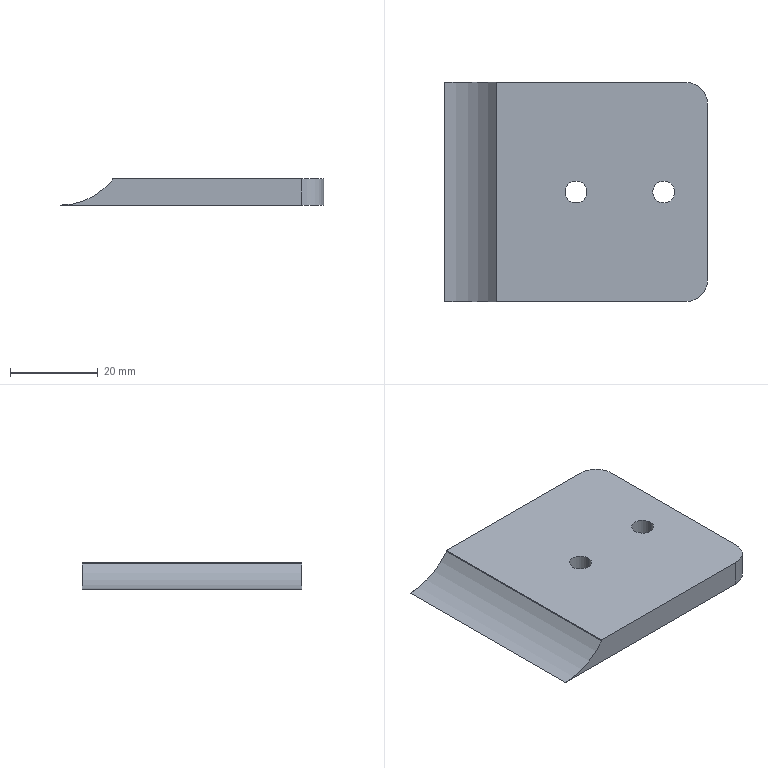Part | SolidWorks | features 3DProfileFeature 1, Extrusion 1, HoleWzd 1, ICE 1 | 1 solid | 13 faces | box 60 x 50 x 6 mm | volume 15185 mm3 | cylinder 7 | plane 6 | commonest cylinder face diameters 5 x4 10 x2 30 x1
STEP:
#1=CARTESIAN_POINT('',(52.5,-30.,-15.));
#2=VERTEX_POINT('',#1);
#3=CARTESIAN_POINT('',(47.5,-30.,-15.));
#4=VERTEX_POINT('',#3);
#5=CARTESIAN_POINT('',(50.,-30.,-15.));
#6=DIRECTION('',(0.,0.,-1.));
#7=DIRECTION('',(-1.,0.,0.));
#8=AXIS2_PLACEMENT_3D('',#5,#6,#7);
#9=CIRCLE('',#8,2.5);
#10=EDGE_CURVE('',#2,#4,#9,.T.);
#11=ORIENTED_EDGE('',*,*,#10,.T.);
#12=CARTESIAN_POINT('',(47.5,-30.,-9.));
#13=VERTEX_POINT('',#12);
#14=CARTESIAN_POINT('',(47.5,-30.,-9.));
#15=DIRECTION('',(0.,0.,1.));
#16=VECTOR('',#15,1000.);
#17=LINE('',#14,#16);
#18=EDGE_CURVE('',#4,#13,#17,.T.);
#19=ORIENTED_EDGE('',*,*,#18,.T.);
#20=CARTESIAN_POINT('',(52.5,-30.,-9.));
#21=VERTEX_POINT('',#20);
#22=CARTESIAN_POINT('',(50.,-30.,-9.));
#23=DIRECTION('',(0.,0.,1.));
#24=DIRECTION('',(1.,0.,0.));
#25=AXIS2_PLACEMENT_3D('',#22,#23,#24);
#26=CIRCLE('',#25,2.5);
#27=EDGE_CURVE('',#13,#21,#26,.T.);
#28=ORIENTED_EDGE('',*,*,#27,.T.);
#29=CARTESIAN_POINT('',(52.5,-30.,-9.));
#30=DIRECTION('',(0.,0.,1.));
#31=VECTOR('',#30,1000.);
#32=LINE('',#29,#31);
#33=EDGE_CURVE('',#2,#21,#32,.T.);
#34=ORIENTED_EDGE('',*,*,#33,.F.);
#35=EDGE_LOOP('',(#11,#19,#28,#34));
#36=FACE_OUTER_BOUND('',#35,.T.);
#37=CARTESIAN_POINT('',(50.,-30.,-9.));
#38=DIRECTION('',(0.,0.,1.));
#39=DIRECTION('',(1.,0.,0.));
#40=AXIS2_PLACEMENT_3D('',#37,#38,#39);
#41=CYLINDRICAL_SURFACE('',#40,2.5);
#42=ADVANCED_FACE('',(#36),#41,.F.);
#43=CARTESIAN_POINT('',(32.5,-30.,-15.));
#44=VERTEX_POINT('',#43);
#45=CARTESIAN_POINT('',(27.5,-30.,-15.));
#46=VERTEX_POINT('',#45);
#47=CARTESIAN_POINT('',(30.,-30.,-15.));
#48=DIRECTION('',(0.,0.,-1.));
#49=DIRECTION('',(-1.,0.,0.));
#50=AXIS2_PLACEMENT_3D('',#47,#48,#49);
#51=CIRCLE('',#50,2.5);
#52=EDGE_CURVE('',#44,#46,#51,.T.);
#53=ORIENTED_EDGE('',*,*,#52,.T.);
#54=CARTESIAN_POINT('',(27.5,-30.,-9.));
#55=VERTEX_POINT('',#54);
#56=CARTESIAN_POINT('',(27.5,-30.,-9.));
#57=DIRECTION('',(0.,0.,1.));
#58=VECTOR('',#57,1000.);
#59=LINE('',#56,#58);
#60=EDGE_CURVE('',#46,#55,#59,.T.);
#61=ORIENTED_EDGE('',*,*,#60,.T.);
#62=CARTESIAN_POINT('',(32.5,-30.,-9.));
#63=VERTEX_POINT('',#62);
#64=CARTESIAN_POINT('',(30.,-30.,-9.));
#65=DIRECTION('',(0.,0.,1.));
#66=DIRECTION('',(1.,0.,0.));
#67=AXIS2_PLACEMENT_3D('',#64,#65,#66);
#68=CIRCLE('',#67,2.5);
#69=EDGE_CURVE('',#55,#63,#68,.T.);
#70=ORIENTED_EDGE('',*,*,#69,.T.);
#71=CARTESIAN_POINT('',(32.5,-30.,-9.));
#72=DIRECTION('',(0.,0.,1.));
#73=VECTOR('',#72,1000.);
#74=LINE('',#71,#73);
#75=EDGE_CURVE('',#44,#63,#74,.T.);
#76=ORIENTED_EDGE('',*,*,#75,.F.);
#77=EDGE_LOOP('',(#53,#61,#70,#76));
#78=FACE_OUTER_BOUND('',#77,.T.);
#79=CARTESIAN_POINT('',(30.,-30.,-9.));
#80=DIRECTION('',(0.,0.,1.));
#81=DIRECTION('',(1.,0.,0.));
#82=AXIS2_PLACEMENT_3D('',#79,#80,#81);
#83=CYLINDRICAL_SURFACE('',#82,2.5);
#84=ADVANCED_FACE('',(#78),#83,.F.);
#85=CARTESIAN_POINT('',(11.8,-55.,-9.261));
#86=VERTEX_POINT('',#85);
#87=CARTESIAN_POINT('',(11.8,-5.,-9.261));
#88=VERTEX_POINT('',#87);
#89=CARTESIAN_POINT('',(11.8,-68.122,-9.261));
#90=DIRECTION('',(0.,1.,0.));
#91=VECTOR('',#90,1000.);
#92=LINE('',#89,#91);
#93=EDGE_CURVE('',#86,#88,#92,.T.);
#94=ORIENTED_EDGE('',*,*,#93,.F.);
#95=CARTESIAN_POINT('',(11.8,-55.,-9.));
#96=VERTEX_POINT('',#95);
#97=CARTESIAN_POINT('',(11.8,-55.,-9.));
#98=DIRECTION('',(0.,0.,-1.));
#99=VECTOR('',#98,1000.);
#100=LINE('',#97,#99);
#101=EDGE_CURVE('',#96,#86,#100,.T.);
#102=ORIENTED_EDGE('',*,*,#101,.F.);
#103=CARTESIAN_POINT('',(11.8,-5.,-9.));
#104=VERTEX_POINT('',#103);
#105=CARTESIAN_POINT('',(11.8,-5.,-9.));
#106=DIRECTION('',(0.,-1.,0.));
#107=VECTOR('',#106,1000.);
#108=LINE('',#105,#107);
#109=EDGE_CURVE('',#104,#96,#108,.T.);
#110=ORIENTED_EDGE('',*,*,#109,.F.);
#111=CARTESIAN_POINT('',(11.8,-5.,-9.));
#112=DIRECTION('',(0.,0.,-1.));
#113=VECTOR('',#112,1000.);
#114=LINE('',#111,#113);
#115=EDGE_CURVE('',#104,#88,#114,.T.);
#116=ORIENTED_EDGE('',*,*,#115,.T.);
#117=EDGE_LOOP('',(#94,#102,#110,#116));
#118=FACE_OUTER_BOUND('',#117,.T.);
#119=CARTESIAN_POINT('',(11.8,-5.,-9.));
#120=DIRECTION('',(1.,0.,0.));
#121=DIRECTION('',(0.,1.,0.));
#122=AXIS2_PLACEMENT_3D('',#119,#120,#121);
#123=PLANE('',#122);
#124=ADVANCED_FACE('',(#118),#123,.F.);
#125=CARTESIAN_POINT('',(0.,-55.,-15.));
#126=VERTEX_POINT('',#125);
#127=CARTESIAN_POINT('',(55.,-55.,-15.));
#128=VERTEX_POINT('',#127);
#129=CARTESIAN_POINT('',(11.8,-55.,-15.));
#130=DIRECTION('',(1.,0.,0.));
#131=VECTOR('',#130,1000.);
#132=LINE('',#129,#131);
#133=EDGE_CURVE('',#126,#128,#132,.T.);
#134=ORIENTED_EDGE('',*,*,#133,.T.);
#135=CARTESIAN_POINT('',(55.,-55.,-9.));
#136=VERTEX_POINT('',#135);
#137=CARTESIAN_POINT('',(55.,-55.,-9.));
#138=DIRECTION('',(0.,0.,-1.));
#139=VECTOR('',#138,1000.);
#140=LINE('',#137,#139);
#141=EDGE_CURVE('',#136,#128,#140,.T.);
#142=ORIENTED_EDGE('',*,*,#141,.F.);
#143=CARTESIAN_POINT('',(11.8,-55.,-9.));
#144=DIRECTION('',(1.,0.,0.));
#145=VECTOR('',#144,1000.);
#146=LINE('',#143,#145);
#147=EDGE_CURVE('',#96,#136,#146,.T.);
#148=ORIENTED_EDGE('',*,*,#147,.F.);
#149=ORIENTED_EDGE('',*,*,#101,.T.);
#150=CARTESIAN_POINT('',(0.,-55.,0.));
#151=DIRECTION('',(0.,1.,0.));
#152=DIRECTION('',(0.,0.,1.));
#153=AXIS2_PLACEMENT_3D('',#150,#151,#152);
#154=CIRCLE('',#153,15.);
#155=EDGE_CURVE('',#86,#126,#154,.T.);
#156=ORIENTED_EDGE('',*,*,#155,.T.);
#157=EDGE_LOOP('',(#134,#142,#148,#149,#156));
#158=FACE_OUTER_BOUND('',#157,.T.);
#159=CARTESIAN_POINT('',(11.8,-55.,-9.));
#160=DIRECTION('',(0.,1.,0.));
#161=DIRECTION('',(0.,0.,1.));
#162=AXIS2_PLACEMENT_3D('',#159,#160,#161);
#163=PLANE('',#162);
#164=ADVANCED_FACE('',(#158),#163,.F.);
#165=CARTESIAN_POINT('',(60.,-50.,-15.));
#166=VERTEX_POINT('',#165);
#167=CARTESIAN_POINT('',(55.,-50.,-15.));
#168=DIRECTION('',(0.,0.,1.));
#169=DIRECTION('',(-1.,0.,0.));
#170=AXIS2_PLACEMENT_3D('',#167,#168,#169);
#171=CIRCLE('',#170,5.);
#172=EDGE_CURVE('',#128,#166,#171,.T.);
#173=ORIENTED_EDGE('',*,*,#172,.T.);
#174=CARTESIAN_POINT('',(60.,-50.,-9.));
#175=VERTEX_POINT('',#174);
#176=CARTESIAN_POINT('',(60.,-50.,-9.));
#177=DIRECTION('',(0.,0.,-1.));
#178=VECTOR('',#177,1000.);
#179=LINE('',#176,#178);
#180=EDGE_CURVE('',#175,#166,#179,.T.);
#181=ORIENTED_EDGE('',*,*,#180,.F.);
#182=CARTESIAN_POINT('',(55.,-50.,-9.));
#183=DIRECTION('',(0.,0.,1.));
#184=DIRECTION('',(-1.,0.,0.));
#185=AXIS2_PLACEMENT_3D('',#182,#183,#184);
#186=CIRCLE('',#185,5.);
#187=EDGE_CURVE('',#136,#175,#186,.T.);
#188=ORIENTED_EDGE('',*,*,#187,.F.);
#189=ORIENTED_EDGE('',*,*,#141,.T.);
#190=EDGE_LOOP('',(#173,#181,#188,#189));
#191=FACE_OUTER_BOUND('',#190,.T.);
#192=CARTESIAN_POINT('',(55.,-50.,-9.));
#193=DIRECTION('',(0.,0.,-1.));
#194=DIRECTION('',(-1.,0.,0.));
#195=AXIS2_PLACEMENT_3D('',#192,#193,#194);
#196=CYLINDRICAL_SURFACE('',#195,5.);
#197=ADVANCED_FACE('',(#191),#196,.T.);
#198=CARTESIAN_POINT('',(60.,-10.,-15.));
#199=VERTEX_POINT('',#198);
#200=CARTESIAN_POINT('',(60.,-10.,-15.));
#201=DIRECTION('',(0.,1.,0.));
#202=VECTOR('',#201,1000.);
#203=LINE('',#200,#202);
#204=EDGE_CURVE('',#166,#199,#203,.T.);
#205=ORIENTED_EDGE('',*,*,#204,.T.);
#206=CARTESIAN_POINT('',(60.,-10.,-9.));
#207=VERTEX_POINT('',#206);
#208=CARTESIAN_POINT('',(60.,-10.,-9.));
#209=DIRECTION('',(0.,0.,-1.));
#210=VECTOR('',#209,1000.);
#211=LINE('',#208,#210);
#212=EDGE_CURVE('',#207,#199,#211,.T.);
#213=ORIENTED_EDGE('',*,*,#212,.F.);
#214=CARTESIAN_POINT('',(60.,-10.,-9.));
#215=DIRECTION('',(0.,1.,0.));
#216=VECTOR('',#215,1000.);
#217=LINE('',#214,#216);
#218=EDGE_CURVE('',#175,#207,#217,.T.);
#219=ORIENTED_EDGE('',*,*,#218,.F.);
#220=ORIENTED_EDGE('',*,*,#180,.T.);
#221=EDGE_LOOP('',(#205,#213,#219,#220));
#222=FACE_OUTER_BOUND('',#221,.T.);
#223=CARTESIAN_POINT('',(60.,-10.,-9.));
#224=DIRECTION('',(-1.,0.,0.));
#225=DIRECTION('',(0.,-1.,0.));
#226=AXIS2_PLACEMENT_3D('',#223,#224,#225);
#227=PLANE('',#226);
#228=ADVANCED_FACE('',(#222),#227,.F.);
#229=CARTESIAN_POINT('',(55.,-5.,-15.));
#230=VERTEX_POINT('',#229);
#231=CARTESIAN_POINT('',(55.,-10.,-15.));
#232=DIRECTION('',(0.,0.,1.));
#233=DIRECTION('',(-1.,0.,0.));
#234=AXIS2_PLACEMENT_3D('',#231,#232,#233);
#235=CIRCLE('',#234,5.);
#236=EDGE_CURVE('',#199,#230,#235,.T.);
#237=ORIENTED_EDGE('',*,*,#236,.T.);
#238=CARTESIAN_POINT('',(55.,-5.,-9.));
#239=VERTEX_POINT('',#238);
#240=CARTESIAN_POINT('',(55.,-5.,-9.));
#241=DIRECTION('',(0.,0.,-1.));
#242=VECTOR('',#241,1000.);
#243=LINE('',#240,#242);
#244=EDGE_CURVE('',#239,#230,#243,.T.);
#245=ORIENTED_EDGE('',*,*,#244,.F.);
#246=CARTESIAN_POINT('',(55.,-10.,-9.));
#247=DIRECTION('',(0.,0.,1.));
#248=DIRECTION('',(-1.,0.,0.));
#249=AXIS2_PLACEMENT_3D('',#246,#247,#248);
#250=CIRCLE('',#249,5.);
#251=EDGE_CURVE('',#207,#239,#250,.T.);
#252=ORIENTED_EDGE('',*,*,#251,.F.);
#253=ORIENTED_EDGE('',*,*,#212,.T.);
#254=EDGE_LOOP('',(#237,#245,#252,#253));
#255=FACE_OUTER_BOUND('',#254,.T.);
#256=CARTESIAN_POINT('',(55.,-10.,-9.));
#257=DIRECTION('',(0.,0.,-1.));
#258=DIRECTION('',(-1.,0.,0.));
#259=AXIS2_PLACEMENT_3D('',#256,#257,#258);
#260=CYLINDRICAL_SURFACE('',#259,5.);
#261=ADVANCED_FACE('',(#255),#260,.T.);
#262=CARTESIAN_POINT('',(0.,-5.,-15.));
#263=VERTEX_POINT('',#262);
#264=CARTESIAN_POINT('',(11.8,-5.,-15.));
#265=DIRECTION('',(-1.,0.,0.));
#266=VECTOR('',#265,1000.);
#267=LINE('',#264,#266);
#268=EDGE_CURVE('',#230,#263,#267,.T.);
#269=ORIENTED_EDGE('',*,*,#268,.T.);
#270=CARTESIAN_POINT('',(0.,-5.,0.));
#271=DIRECTION('',(0.,-1.,0.));
#272=DIRECTION('',(0.,0.,1.));
#273=AXIS2_PLACEMENT_3D('',#270,#271,#272);
#274=CIRCLE('',#273,15.);
#275=EDGE_CURVE('',#263,#88,#274,.T.);
#276=ORIENTED_EDGE('',*,*,#275,.T.);
#277=ORIENTED_EDGE('',*,*,#115,.F.);
#278=CARTESIAN_POINT('',(11.8,-5.,-9.));
#279=DIRECTION('',(-1.,0.,0.));
#280=VECTOR('',#279,1000.);
#281=LINE('',#278,#280);
#282=EDGE_CURVE('',#239,#104,#281,.T.);
#283=ORIENTED_EDGE('',*,*,#282,.F.);
#284=ORIENTED_EDGE('',*,*,#244,.T.);
#285=EDGE_LOOP('',(#269,#276,#277,#283,#284));
#286=FACE_OUTER_BOUND('',#285,.T.);
#287=CARTESIAN_POINT('',(11.8,-5.,-9.));
#288=DIRECTION('',(0.,-1.,0.));
#289=DIRECTION('',(0.,0.,-1.));
#290=AXIS2_PLACEMENT_3D('',#287,#288,#289);
#291=PLANE('',#290);
#292=ADVANCED_FACE('',(#286),#291,.F.);
#293=CARTESIAN_POINT('',(50.,-30.,-9.));
#294=DIRECTION('',(0.,0.,1.));
#295=DIRECTION('',(1.,0.,0.));
#296=AXIS2_PLACEMENT_3D('',#293,#294,#295);
#297=CIRCLE('',#296,2.5);
#298=EDGE_CURVE('',#21,#13,#297,.T.);
#299=ORIENTED_EDGE('',*,*,#298,.F.);
#300=ORIENTED_EDGE('',*,*,#27,.F.);
#301=EDGE_LOOP('',(#299,#300));
#302=FACE_BOUND('',#301,.T.);
#303=CARTESIAN_POINT('',(30.,-30.,-9.));
#304=DIRECTION('',(0.,0.,1.));
#305=DIRECTION('',(1.,0.,0.));
#306=AXIS2_PLACEMENT_3D('',#303,#304,#305);
#307=CIRCLE('',#306,2.5);
#308=EDGE_CURVE('',#63,#55,#307,.T.);
#309=ORIENTED_EDGE('',*,*,#308,.F.);
#310=ORIENTED_EDGE('',*,*,#69,.F.);
#311=EDGE_LOOP('',(#309,#310));
#312=FACE_BOUND('',#311,.T.);
#313=ORIENTED_EDGE('',*,*,#109,.T.);
#314=ORIENTED_EDGE('',*,*,#147,.T.);
#315=ORIENTED_EDGE('',*,*,#187,.T.);
#316=ORIENTED_EDGE('',*,*,#218,.T.);
#317=ORIENTED_EDGE('',*,*,#251,.T.);
#318=ORIENTED_EDGE('',*,*,#282,.T.);
#319=EDGE_LOOP('',(#313,#314,#315,#316,#317,#318));
#320=FACE_OUTER_BOUND('',#319,.T.);
#321=CARTESIAN_POINT('',(55.,-50.,-9.));
#322=DIRECTION('',(0.,0.,-1.));
#323=DIRECTION('',(-1.,0.,0.));
#324=AXIS2_PLACEMENT_3D('',#321,#322,#323);
#325=PLANE('',#324);
#326=ADVANCED_FACE('',(#302,#312,#320),#325,.F.);
#327=ORIENTED_EDGE('',*,*,#10,.F.);
#328=CARTESIAN_POINT('',(50.,-30.,-15.));
#329=DIRECTION('',(0.,0.,-1.));
#330=DIRECTION('',(-1.,0.,0.));
#331=AXIS2_PLACEMENT_3D('',#328,#329,#330);
#332=CIRCLE('',#331,2.5);
#333=EDGE_CURVE('',#4,#2,#332,.T.);
#334=ORIENTED_EDGE('',*,*,#333,.F.);
#335=EDGE_LOOP('',(#327,#334));
#336=FACE_BOUND('',#335,.T.);
#337=ORIENTED_EDGE('',*,*,#52,.F.);
#338=CARTESIAN_POINT('',(30.,-30.,-15.));
#339=DIRECTION('',(0.,0.,-1.));
#340=DIRECTION('',(-1.,0.,0.));
#341=AXIS2_PLACEMENT_3D('',#338,#339,#340);
#342=CIRCLE('',#341,2.5);
#343=EDGE_CURVE('',#46,#44,#342,.T.);
#344=ORIENTED_EDGE('',*,*,#343,.F.);
#345=EDGE_LOOP('',(#337,#344));
#346=FACE_BOUND('',#345,.T.);
#347=ORIENTED_EDGE('',*,*,#133,.F.);
#348=CARTESIAN_POINT('',(0.,-68.122,-15.));
#349=DIRECTION('',(0.,1.,0.));
#350=VECTOR('',#349,1000.);
#351=LINE('',#348,#350);
#352=EDGE_CURVE('',#126,#263,#351,.T.);
#353=ORIENTED_EDGE('',*,*,#352,.T.);
#354=ORIENTED_EDGE('',*,*,#268,.F.);
#355=ORIENTED_EDGE('',*,*,#236,.F.);
#356=ORIENTED_EDGE('',*,*,#204,.F.);
#357=ORIENTED_EDGE('',*,*,#172,.F.);
#358=EDGE_LOOP('',(#347,#353,#354,#355,#356,#357));
#359=FACE_OUTER_BOUND('',#358,.T.);
#360=CARTESIAN_POINT('',(55.,-50.,-15.));
#361=DIRECTION('',(0.,0.,-1.));
#362=DIRECTION('',(-1.,0.,0.));
#363=AXIS2_PLACEMENT_3D('',#360,#361,#362);
#364=PLANE('',#363);
#365=ADVANCED_FACE('',(#336,#346,#359),#364,.T.);
#366=ORIENTED_EDGE('',*,*,#155,.F.);
#367=ORIENTED_EDGE('',*,*,#93,.T.);
#368=ORIENTED_EDGE('',*,*,#275,.F.);
#369=ORIENTED_EDGE('',*,*,#352,.F.);
#370=EDGE_LOOP('',(#366,#367,#368,#369));
#371=FACE_OUTER_BOUND('',#370,.T.);
#372=CARTESIAN_POINT('',(0.,-68.122,0.));
#373=DIRECTION('',(0.,1.,0.));
#374=DIRECTION('',(0.,0.,1.));
#375=AXIS2_PLACEMENT_3D('',#372,#373,#374);
#376=CYLINDRICAL_SURFACE('',#375,15.);
#377=ADVANCED_FACE('',(#371),#376,.F.);
#378=ORIENTED_EDGE('',*,*,#60,.F.);
#379=ORIENTED_EDGE('',*,*,#343,.T.);
#380=ORIENTED_EDGE('',*,*,#75,.T.);
#381=ORIENTED_EDGE('',*,*,#308,.T.);
#382=EDGE_LOOP('',(#378,#379,#380,#381));
#383=FACE_OUTER_BOUND('',#382,.T.);
#384=CARTESIAN_POINT('',(30.,-30.,-9.));
#385=DIRECTION('',(0.,0.,1.));
#386=DIRECTION('',(1.,0.,0.));
#387=AXIS2_PLACEMENT_3D('',#384,#385,#386);
#388=CYLINDRICAL_SURFACE('',#387,2.5);
#389=ADVANCED_FACE('',(#383),#388,.F.);
#390=ORIENTED_EDGE('',*,*,#18,.F.);
#391=ORIENTED_EDGE('',*,*,#333,.T.);
#392=ORIENTED_EDGE('',*,*,#33,.T.);
#393=ORIENTED_EDGE('',*,*,#298,.T.);
#394=EDGE_LOOP('',(#390,#391,#392,#393));
#395=FACE_OUTER_BOUND('',#394,.T.);
#396=CARTESIAN_POINT('',(50.,-30.,-9.));
#397=DIRECTION('',(0.,0.,1.));
#398=DIRECTION('',(1.,0.,0.));
#399=AXIS2_PLACEMENT_3D('',#396,#397,#398);
#400=CYLINDRICAL_SURFACE('',#399,2.5);
#401=ADVANCED_FACE('',(#395),#400,.F.);
#402=CLOSED_SHELL('',(#42,#84,#124,#164,#197,#228,#261,#292,#326,#365,#377,#389,#401));
#403=MANIFOLD_SOLID_BREP('',#402);
#404=CARTESIAN_POINT('',(0.,0.,0.));
#405=DIRECTION('',(0.,0.,1.));
#406=DIRECTION('',(1.,0.,0.));
#407=AXIS2_PLACEMENT_3D('',#404,#405,#406);
#408=(LENGTH_UNIT()NAMED_UNIT(*)SI_UNIT(.MILLI.,.METRE.));
#409=UNCERTAINTY_MEASURE_WITH_UNIT(LENGTH_MEASURE(0.00001),#408,'','');
#410=(NAMED_UNIT(*)PLANE_ANGLE_UNIT()SI_UNIT($,.RADIAN.));
#411=(NAMED_UNIT(*)SI_UNIT($,.STERADIAN.)SOLID_ANGLE_UNIT());
#412=(GEOMETRIC_REPRESENTATION_CONTEXT(3)GLOBAL_UNCERTAINTY_ASSIGNED_CONTEXT((#409))GLOBAL_UNIT_ASSIGNED_CONTEXT((#408,#410,#411))REPRESENTATION_CONTEXT('',''));
#413=ADVANCED_BREP_SHAPE_REPRESENTATION('',(#403,#407),#412);